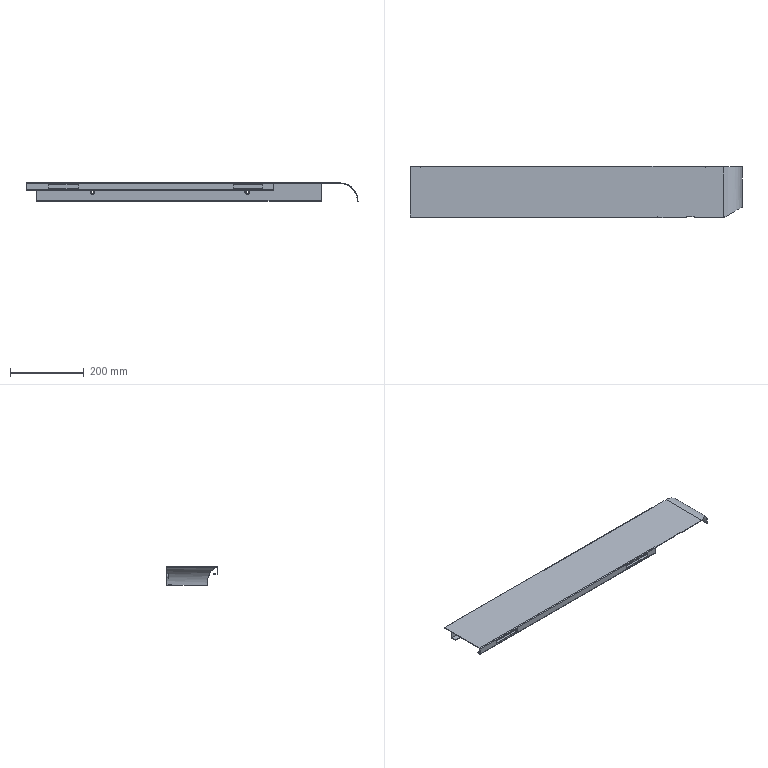Part | STEP file | FHD-021-001-F rack welded part F | 1 solid | 55 faces | box 900 x 139 x 50 mm | volume 288308 mm3 | plane 40 | cylinder 14 | spline 1 | commonest cylinder face diameters 0.4 x4 3.4 x4 6.8 x2 13 x2 97 x1 100 x1